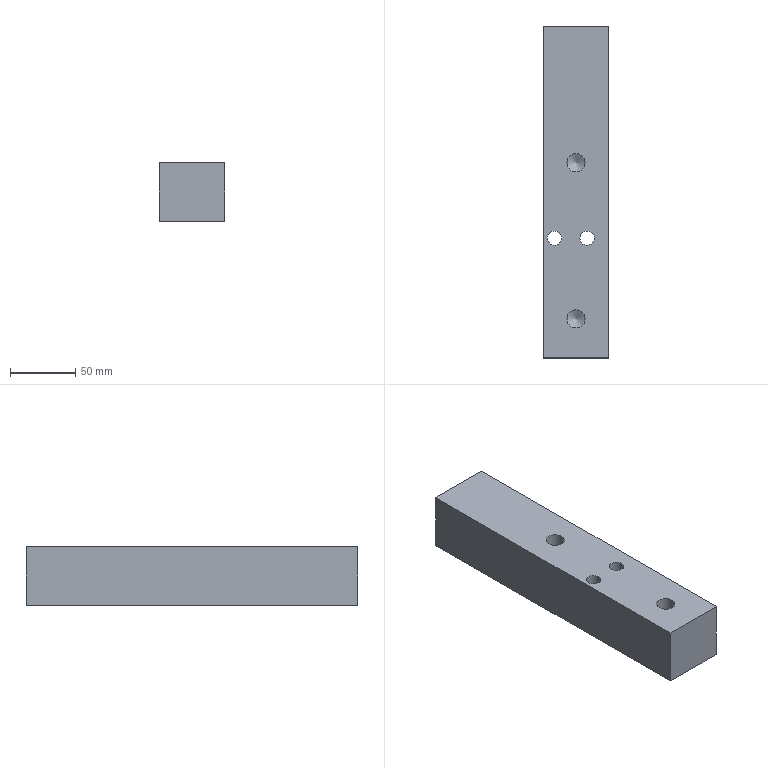Part | STEP file | 019_id2166_x_t | 1 solid | 14 faces | box 50 x 255 x 45 mm | volume 554819 mm3 | plane 6 | cylinder 5 | cone 3 | commonest cylinder face diameters 14 x3 11 x2
STEP:
#1=CARTESIAN_POINT('',(0.,0.,0.));
#2=DIRECTION('',(0.,0.,1.));
#3=DIRECTION('',(1.,0.,0.));
#4=AXIS2_PLACEMENT_3D('',#1,#2,#3);
#5=CARTESIAN_POINT('',(7.5,232.,185.));
#6=VERTEX_POINT('',#5);
#7=CARTESIAN_POINT('',(-3.5,232.,185.));
#8=VERTEX_POINT('',#7);
#9=CARTESIAN_POINT('',(2.,232.,185.));
#10=DIRECTION('',(0.,0.,1.));
#11=DIRECTION('',(1.,0.,0.));
#12=AXIS2_PLACEMENT_3D('',#9,#10,#11);
#13=CIRCLE('',#12,5.5);
#14=CARTESIAN_POINT('',(173.5,0.,185.));
#15=DIRECTION('',(0.,0.,-1.));
#16=DIRECTION('',(1.,0.,0.));
#17=AXIS2_PLACEMENT_3D('',#14,#15,#16);
#18=PLANE('',#17);
#19=CARTESIAN_POINT('',(-166.,-232.));
#20=CARTESIAN_POINT('',(-166.,-241.526));
#21=CARTESIAN_POINT('',(-174.25,-236.763));
#22=CARTESIAN_POINT('',(-182.5,-232.));
#23=CARTESIAN_POINT('',(-174.25,-227.237));
#24=CARTESIAN_POINT('',(-166.,-222.474));
#25=CARTESIAN_POINT('',(-166.,-232.));
#26=(BOUNDED_CURVE()B_SPLINE_CURVE(2,(#19,#20,#21,#22,#23,#24,#25),.UNSPECIFIED.,.T.,.F.)B_SPLINE_CURVE_WITH_KNOTS((1,2,2,2,2,1),(-2.094,0.,2.094,4.189,6.283,8.378),.UNSPECIFIED.)CURVE()GEOMETRIC_REPRESENTATION_ITEM()RATIONAL_B_SPLINE_CURVE((1.,0.5,1.,0.5,1.,0.5,1.))REPRESENTATION_ITEM(''));
#27=(GEOMETRIC_REPRESENTATION_CONTEXT(2)PARAMETRIC_REPRESENTATION_CONTEXT()REPRESENTATION_CONTEXT('',''));
#28=DEFINITIONAL_REPRESENTATION('',(#26),#27);
#29=PCURVE('',#18,#28);
#30=CARTESIAN_POINT('',(2.,232.,595.));
#31=DIRECTION('',(0.,0.,-1.));
#32=DIRECTION('',(-1.,0.,0.));
#33=AXIS2_PLACEMENT_3D('',#30,#31,#32);
#34=CYLINDRICAL_SURFACE('',#33,5.5);
#35=CARTESIAN_POINT('',(3.142,410.));
#36=DIRECTION('',(-1.,0.));
#37=VECTOR('',#36,1.);
#38=LINE('',#35,#37);
#39=(GEOMETRIC_REPRESENTATION_CONTEXT(2)PARAMETRIC_REPRESENTATION_CONTEXT()REPRESENTATION_CONTEXT('',''));
#40=DEFINITIONAL_REPRESENTATION('',(#38),#39);
#41=PCURVE('',#34,#40);
#42=SURFACE_CURVE('',#13,(#29,#41),.PCURVE_S1.);
#43=EDGE_CURVE('',#6,#8,#42,.T.);
#44=ORIENTED_EDGE('',*,*,#43,.T.);
#45=CARTESIAN_POINT('',(2.,232.,185.));
#46=DIRECTION('',(0.,0.,1.));
#47=DIRECTION('',(1.,0.,0.));
#48=AXIS2_PLACEMENT_3D('',#45,#46,#47);
#49=CIRCLE('',#48,5.5);
#50=CARTESIAN_POINT('',(-166.,-232.));
#51=CARTESIAN_POINT('',(-166.,-241.526));
#52=CARTESIAN_POINT('',(-174.25,-236.763));
#53=CARTESIAN_POINT('',(-182.5,-232.));
#54=CARTESIAN_POINT('',(-174.25,-227.237));
#55=CARTESIAN_POINT('',(-166.,-222.474));
#56=CARTESIAN_POINT('',(-166.,-232.));
#57=(BOUNDED_CURVE()B_SPLINE_CURVE(2,(#50,#51,#52,#53,#54,#55,#56),.UNSPECIFIED.,.T.,.F.)B_SPLINE_CURVE_WITH_KNOTS((1,2,2,2,2,1),(-2.094,0.,2.094,4.189,6.283,8.378),.UNSPECIFIED.)CURVE()GEOMETRIC_REPRESENTATION_ITEM()RATIONAL_B_SPLINE_CURVE((1.,0.5,1.,0.5,1.,0.5,1.))REPRESENTATION_ITEM(''));
#58=(GEOMETRIC_REPRESENTATION_CONTEXT(2)PARAMETRIC_REPRESENTATION_CONTEXT()REPRESENTATION_CONTEXT('',''));
#59=DEFINITIONAL_REPRESENTATION('',(#57),#58);
#60=PCURVE('',#18,#59);
#61=CARTESIAN_POINT('',(9.425,410.));
#62=DIRECTION('',(-1.,0.));
#63=VECTOR('',#62,1.);
#64=LINE('',#61,#63);
#65=(GEOMETRIC_REPRESENTATION_CONTEXT(2)PARAMETRIC_REPRESENTATION_CONTEXT()REPRESENTATION_CONTEXT('',''));
#66=DEFINITIONAL_REPRESENTATION('',(#64),#65);
#67=PCURVE('',#34,#66);
#68=SURFACE_CURVE('',#49,(#60,#67),.PCURVE_S1.);
#69=EDGE_CURVE('',#8,#6,#68,.T.);
#70=ORIENTED_EDGE('',*,*,#69,.T.);
#71=EDGE_LOOP('',(#44,#70));
#72=FACE_BOUND('',#71,.T.);
#73=CARTESIAN_POINT('',(-13.5,370.,185.));
#74=VERTEX_POINT('',#73);
#75=CARTESIAN_POINT('',(-6.5,370.,185.));
#76=DIRECTION('',(0.,0.,-1.));
#77=DIRECTION('',(-1.,0.,0.));
#78=AXIS2_PLACEMENT_3D('',#75,#76,#77);
#79=CIRCLE('',#78,7.);
#80=CARTESIAN_POINT('',(-180.,-370.));
#81=DIRECTION('',(-1.,0.));
#82=AXIS2_PLACEMENT_2D('',#80,#81);
#83=CIRCLE('',#82,7.);
#84=(GEOMETRIC_REPRESENTATION_CONTEXT(2)PARAMETRIC_REPRESENTATION_CONTEXT()REPRESENTATION_CONTEXT('',''));
#85=DEFINITIONAL_REPRESENTATION('',(#83),#84);
#86=PCURVE('',#18,#85);
#87=CARTESIAN_POINT('',(-6.5,370.,121.));
#88=DIRECTION('',(0.,0.,1.));
#89=DIRECTION('',(1.,0.,0.));
#90=AXIS2_PLACEMENT_3D('',#87,#88,#89);
#91=CYLINDRICAL_SURFACE('',#90,7.);
#92=CARTESIAN_POINT('',(9.425,64.));
#93=DIRECTION('',(-1.,0.));
#94=VECTOR('',#93,1.);
#95=LINE('',#92,#94);
#96=(GEOMETRIC_REPRESENTATION_CONTEXT(2)PARAMETRIC_REPRESENTATION_CONTEXT()REPRESENTATION_CONTEXT('',''));
#97=DEFINITIONAL_REPRESENTATION('',(#95),#96);
#98=PCURVE('',#91,#97);
#99=SURFACE_CURVE('',#79,(#86,#98),.PCURVE_S1.);
#100=EDGE_CURVE('',#74,#74,#99,.T.);
#101=ORIENTED_EDGE('',*,*,#100,.F.);
#102=EDGE_LOOP('',(#101));
#103=FACE_BOUND('',#102,.T.);
#104=CARTESIAN_POINT('',(18.5,395.,185.));
#105=VERTEX_POINT('',#104);
#106=CARTESIAN_POINT('',(18.5,140.,185.));
#107=VERTEX_POINT('',#106);
#108=CARTESIAN_POINT('',(18.5,-210.,185.));
#109=DIRECTION('',(0.,-1.,0.));
#110=VECTOR('',#109,1.);
#111=LINE('',#108,#110);
#112=CARTESIAN_POINT('',(-155.,210.));
#113=DIRECTION('',(0.,1.));
#114=VECTOR('',#113,1.);
#115=LINE('',#112,#114);
#116=(GEOMETRIC_REPRESENTATION_CONTEXT(2)PARAMETRIC_REPRESENTATION_CONTEXT()REPRESENTATION_CONTEXT('',''));
#117=DEFINITIONAL_REPRESENTATION('',(#115),#116);
#118=PCURVE('',#18,#117);
#119=CARTESIAN_POINT('',(18.5,-210.,-28.5));
#120=DIRECTION('',(-1.,0.,0.));
#121=DIRECTION('',(0.,0.,1.));
#122=AXIS2_PLACEMENT_3D('',#119,#120,#121);
#123=PLANE('',#122);
#124=CARTESIAN_POINT('',(213.5,0.));
#125=DIRECTION('',(0.,-1.));
#126=VECTOR('',#125,1.);
#127=LINE('',#124,#126);
#128=(GEOMETRIC_REPRESENTATION_CONTEXT(2)PARAMETRIC_REPRESENTATION_CONTEXT()REPRESENTATION_CONTEXT('',''));
#129=DEFINITIONAL_REPRESENTATION('',(#127),#128);
#130=PCURVE('',#123,#129);
#131=SURFACE_CURVE('',#111,(#118,#130),.PCURVE_S1.);
#132=EDGE_CURVE('',#105,#107,#131,.T.);
#133=ORIENTED_EDGE('',*,*,#132,.T.);
#134=CARTESIAN_POINT('',(-31.5,140.,185.));
#135=VERTEX_POINT('',#134);
#136=CARTESIAN_POINT('',(513.5,140.,185.));
#137=DIRECTION('',(-1.,0.,0.));
#138=VECTOR('',#137,1.);
#139=LINE('',#136,#138);
#140=CARTESIAN_POINT('',(340.,-140.));
#141=DIRECTION('',(-1.,0.));
#142=VECTOR('',#141,1.);
#143=LINE('',#140,#142);
#144=(GEOMETRIC_REPRESENTATION_CONTEXT(2)PARAMETRIC_REPRESENTATION_CONTEXT()REPRESENTATION_CONTEXT('',''));
#145=DEFINITIONAL_REPRESENTATION('',(#143),#144);
#146=PCURVE('',#18,#145);
#147=CARTESIAN_POINT('',(513.5,140.,428.5));
#148=DIRECTION('',(0.,1.,0.));
#149=DIRECTION('',(0.,0.,-1.));
#150=AXIS2_PLACEMENT_3D('',#147,#148,#149);
#151=PLANE('',#150);
#152=CARTESIAN_POINT('',(243.5,0.));
#153=DIRECTION('',(0.,1.));
#154=VECTOR('',#153,1.);
#155=LINE('',#152,#154);
#156=(GEOMETRIC_REPRESENTATION_CONTEXT(2)PARAMETRIC_REPRESENTATION_CONTEXT()REPRESENTATION_CONTEXT('',''));
#157=DEFINITIONAL_REPRESENTATION('',(#155),#156);
#158=PCURVE('',#151,#157);
#159=SURFACE_CURVE('',#139,(#146,#158),.PCURVE_S1.);
#160=EDGE_CURVE('',#107,#135,#159,.T.);
#161=ORIENTED_EDGE('',*,*,#160,.T.);
#162=CARTESIAN_POINT('',(-31.5,395.,185.));
#163=VERTEX_POINT('',#162);
#164=CARTESIAN_POINT('',(-31.5,0.,185.));
#165=DIRECTION('',(0.,1.,0.));
#166=VECTOR('',#165,1.);
#167=LINE('',#164,#166);
#168=CARTESIAN_POINT('',(-205.,0.));
#169=DIRECTION('',(0.,-1.));
#170=VECTOR('',#169,1.);
#171=LINE('',#168,#170);
#172=(GEOMETRIC_REPRESENTATION_CONTEXT(2)PARAMETRIC_REPRESENTATION_CONTEXT()REPRESENTATION_CONTEXT('',''));
#173=DEFINITIONAL_REPRESENTATION('',(#171),#172);
#174=PCURVE('',#18,#173);
#175=CARTESIAN_POINT('',(-31.5,-210.,-28.5));
#176=DIRECTION('',(-1.,0.,0.));
#177=DIRECTION('',(0.,0.,1.));
#178=AXIS2_PLACEMENT_3D('',#175,#176,#177);
#179=PLANE('',#178);
#180=CARTESIAN_POINT('',(213.5,210.));
#181=DIRECTION('',(0.,1.));
#182=VECTOR('',#181,1.);
#183=LINE('',#180,#182);
#184=(GEOMETRIC_REPRESENTATION_CONTEXT(2)PARAMETRIC_REPRESENTATION_CONTEXT()REPRESENTATION_CONTEXT('',''));
#185=DEFINITIONAL_REPRESENTATION('',(#183),#184);
#186=PCURVE('',#179,#185);
#187=SURFACE_CURVE('',#167,(#174,#186),.PCURVE_S1.);
#188=EDGE_CURVE('',#135,#163,#187,.T.);
#189=ORIENTED_EDGE('',*,*,#188,.T.);
#190=CARTESIAN_POINT('',(173.5,395.,185.));
#191=DIRECTION('',(1.,0.,0.));
#192=VECTOR('',#191,1.);
#193=LINE('',#190,#192);
#194=CARTESIAN_POINT('',(0.,-395.));
#195=DIRECTION('',(1.,0.));
#196=VECTOR('',#195,1.);
#197=LINE('',#194,#196);
#198=(GEOMETRIC_REPRESENTATION_CONTEXT(2)PARAMETRIC_REPRESENTATION_CONTEXT()REPRESENTATION_CONTEXT('',''));
#199=DEFINITIONAL_REPRESENTATION('',(#197),#198);
#200=PCURVE('',#18,#199);
#201=CARTESIAN_POINT('',(-31.5,395.,-28.5));
#202=DIRECTION('',(0.,1.,0.));
#203=DIRECTION('',(0.,0.,-1.));
#204=AXIS2_PLACEMENT_3D('',#201,#202,#203);
#205=PLANE('',#204);
#206=CARTESIAN_POINT('',(-213.5,-205.));
#207=DIRECTION('',(0.,-1.));
#208=VECTOR('',#207,1.);
#209=LINE('',#206,#208);
#210=(GEOMETRIC_REPRESENTATION_CONTEXT(2)PARAMETRIC_REPRESENTATION_CONTEXT()REPRESENTATION_CONTEXT('',''));
#211=DEFINITIONAL_REPRESENTATION('',(#209),#210);
#212=PCURVE('',#205,#211);
#213=SURFACE_CURVE('',#193,(#200,#212),.PCURVE_S1.);
#214=EDGE_CURVE('',#163,#105,#213,.T.);
#215=ORIENTED_EDGE('',*,*,#214,.T.);
#216=EDGE_LOOP('',(#133,#161,#189,#215));
#217=FACE_BOUND('',#216,.T.);
#218=CARTESIAN_POINT('',(-17.5,232.,185.));
#219=VERTEX_POINT('',#218);
#220=CARTESIAN_POINT('',(-28.5,232.,185.));
#221=VERTEX_POINT('',#220);
#222=CARTESIAN_POINT('',(-23.,232.,185.));
#223=DIRECTION('',(0.,0.,1.));
#224=DIRECTION('',(1.,0.,0.));
#225=AXIS2_PLACEMENT_3D('',#222,#223,#224);
#226=CIRCLE('',#225,5.5);
#227=CARTESIAN_POINT('',(-191.,-232.));
#228=CARTESIAN_POINT('',(-191.,-241.526));
#229=CARTESIAN_POINT('',(-199.25,-236.763));
#230=CARTESIAN_POINT('',(-207.5,-232.));
#231=CARTESIAN_POINT('',(-199.25,-227.237));
#232=CARTESIAN_POINT('',(-191.,-222.474));
#233=CARTESIAN_POINT('',(-191.,-232.));
#234=(BOUNDED_CURVE()B_SPLINE_CURVE(2,(#227,#228,#229,#230,#231,#232,#233),.UNSPECIFIED.,.T.,.F.)B_SPLINE_CURVE_WITH_KNOTS((1,2,2,2,2,1),(-2.094,0.,2.094,4.189,6.283,8.378),.UNSPECIFIED.)CURVE()GEOMETRIC_REPRESENTATION_ITEM()RATIONAL_B_SPLINE_CURVE((1.,0.5,1.,0.5,1.,0.5,1.))REPRESENTATION_ITEM(''));
#235=(GEOMETRIC_REPRESENTATION_CONTEXT(2)PARAMETRIC_REPRESENTATION_CONTEXT()REPRESENTATION_CONTEXT('',''));
#236=DEFINITIONAL_REPRESENTATION('',(#234),#235);
#237=PCURVE('',#18,#236);
#238=CARTESIAN_POINT('',(-23.,232.,595.));
#239=DIRECTION('',(0.,0.,-1.));
#240=DIRECTION('',(-1.,0.,0.));
#241=AXIS2_PLACEMENT_3D('',#238,#239,#240);
#242=CYLINDRICAL_SURFACE('',#241,5.5);
#243=CARTESIAN_POINT('',(3.142,410.));
#244=DIRECTION('',(-1.,0.));
#245=VECTOR('',#244,1.);
#246=LINE('',#243,#245);
#247=(GEOMETRIC_REPRESENTATION_CONTEXT(2)PARAMETRIC_REPRESENTATION_CONTEXT()REPRESENTATION_CONTEXT('',''));
#248=DEFINITIONAL_REPRESENTATION('',(#246),#247);
#249=PCURVE('',#242,#248);
#250=SURFACE_CURVE('',#226,(#237,#249),.PCURVE_S1.);
#251=EDGE_CURVE('',#219,#221,#250,.T.);
#252=ORIENTED_EDGE('',*,*,#251,.T.);
#253=CARTESIAN_POINT('',(-23.,232.,185.));
#254=DIRECTION('',(0.,0.,1.));
#255=DIRECTION('',(1.,0.,0.));
#256=AXIS2_PLACEMENT_3D('',#253,#254,#255);
#257=CIRCLE('',#256,5.5);
#258=CARTESIAN_POINT('',(-191.,-232.));
#259=CARTESIAN_POINT('',(-191.,-241.526));
#260=CARTESIAN_POINT('',(-199.25,-236.763));
#261=CARTESIAN_POINT('',(-207.5,-232.));
#262=CARTESIAN_POINT('',(-199.25,-227.237));
#263=CARTESIAN_POINT('',(-191.,-222.474));
#264=CARTESIAN_POINT('',(-191.,-232.));
#265=(BOUNDED_CURVE()B_SPLINE_CURVE(2,(#258,#259,#260,#261,#262,#263,#264),.UNSPECIFIED.,.T.,.F.)B_SPLINE_CURVE_WITH_KNOTS((1,2,2,2,2,1),(-2.094,0.,2.094,4.189,6.283,8.378),.UNSPECIFIED.)CURVE()GEOMETRIC_REPRESENTATION_ITEM()RATIONAL_B_SPLINE_CURVE((1.,0.5,1.,0.5,1.,0.5,1.))REPRESENTATION_ITEM(''));
#266=(GEOMETRIC_REPRESENTATION_CONTEXT(2)PARAMETRIC_REPRESENTATION_CONTEXT()REPRESENTATION_CONTEXT('',''));
#267=DEFINITIONAL_REPRESENTATION('',(#265),#266);
#268=PCURVE('',#18,#267);
#269=CARTESIAN_POINT('',(9.425,410.));
#270=DIRECTION('',(-1.,0.));
#271=VECTOR('',#270,1.);
#272=LINE('',#269,#271);
#273=(GEOMETRIC_REPRESENTATION_CONTEXT(2)PARAMETRIC_REPRESENTATION_CONTEXT()REPRESENTATION_CONTEXT('',''));
#274=DEFINITIONAL_REPRESENTATION('',(#272),#273);
#275=PCURVE('',#242,#274);
#276=SURFACE_CURVE('',#257,(#268,#275),.PCURVE_S1.);
#277=EDGE_CURVE('',#221,#219,#276,.T.);
#278=ORIENTED_EDGE('',*,*,#277,.T.);
#279=EDGE_LOOP('',(#252,#278));
#280=FACE_BOUND('',#279,.T.);
#281=ADVANCED_FACE('',(#72,#103,#217,#280),#18,.T.);
#282=CARTESIAN_POINT('',(-3.5,232.,230.));
#283=VERTEX_POINT('',#282);
#284=CARTESIAN_POINT('',(2.,232.,230.));
#285=DIRECTION('',(0.,0.,1.));
#286=DIRECTION('',(-1.,0.,0.));
#287=AXIS2_PLACEMENT_3D('',#284,#285,#286);
#288=CIRCLE('',#287,5.5);
#289=CARTESIAN_POINT('',(-31.5,-210.,230.));
#290=DIRECTION('',(0.,0.,-1.));
#291=DIRECTION('',(0.,-1.,0.));
#292=AXIS2_PLACEMENT_3D('',#289,#290,#291);
#293=PLANE('',#292);
#294=CARTESIAN_POINT('',(-442.,-28.));
#295=CARTESIAN_POINT('',(-432.474,-28.));
#296=CARTESIAN_POINT('',(-437.237,-36.25));
#297=CARTESIAN_POINT('',(-442.,-44.5));
#298=CARTESIAN_POINT('',(-446.763,-36.25));
#299=CARTESIAN_POINT('',(-451.526,-28.));
#300=CARTESIAN_POINT('',(-442.,-28.));
#301=(BOUNDED_CURVE()B_SPLINE_CURVE(2,(#294,#295,#296,#297,#298,#299,#300),.UNSPECIFIED.,.T.,.F.)B_SPLINE_CURVE_WITH_KNOTS((1,2,2,2,2,1),(-2.094,0.,2.094,4.189,6.283,8.378),.UNSPECIFIED.)CURVE()GEOMETRIC_REPRESENTATION_ITEM()RATIONAL_B_SPLINE_CURVE((1.,0.5,1.,0.5,1.,0.5,1.))REPRESENTATION_ITEM(''));
#302=(GEOMETRIC_REPRESENTATION_CONTEXT(2)PARAMETRIC_REPRESENTATION_CONTEXT()REPRESENTATION_CONTEXT('',''));
#303=DEFINITIONAL_REPRESENTATION('',(#301),#302);
#304=PCURVE('',#293,#303);
#305=CARTESIAN_POINT('',(6.283,365.));
#306=DIRECTION('',(-1.,0.));
#307=VECTOR('',#306,1.);
#308=LINE('',#305,#307);
#309=(GEOMETRIC_REPRESENTATION_CONTEXT(2)PARAMETRIC_REPRESENTATION_CONTEXT()REPRESENTATION_CONTEXT('',''));
#310=DEFINITIONAL_REPRESENTATION('',(#308),#309);
#311=PCURVE('',#34,#310);
#312=SURFACE_CURVE('',#288,(#304,#311),.PCURVE_S1.);
#313=EDGE_CURVE('',#283,#283,#312,.T.);
#314=ORIENTED_EDGE('',*,*,#313,.F.);
#315=EDGE_LOOP('',(#314));
#316=FACE_BOUND('',#315,.T.);
#317=CARTESIAN_POINT('',(-13.5,170.,230.));
#318=VERTEX_POINT('',#317);
#319=CARTESIAN_POINT('',(-6.5,170.,230.));
#320=DIRECTION('',(0.,0.,-1.));
#321=DIRECTION('',(-1.,0.,0.));
#322=AXIS2_PLACEMENT_3D('',#319,#320,#321);
#323=CIRCLE('',#322,7.);
#324=CARTESIAN_POINT('',(-380.,-25.));
#325=DIRECTION('',(0.,1.));
#326=AXIS2_PLACEMENT_2D('',#324,#325);
#327=CIRCLE('',#326,7.);
#328=(GEOMETRIC_REPRESENTATION_CONTEXT(2)PARAMETRIC_REPRESENTATION_CONTEXT()REPRESENTATION_CONTEXT('',''));
#329=DEFINITIONAL_REPRESENTATION('',(#327),#328);
#330=PCURVE('',#293,#329);
#331=CARTESIAN_POINT('',(-6.5,170.,279.));
#332=DIRECTION('',(0.,0.,-1.));
#333=DIRECTION('',(1.,0.,0.));
#334=AXIS2_PLACEMENT_3D('',#331,#332,#333);
#335=CYLINDRICAL_SURFACE('',#334,7.);
#336=CARTESIAN_POINT('',(3.142,49.));
#337=DIRECTION('',(1.,0.));
#338=VECTOR('',#337,1.);
#339=LINE('',#336,#338);
#340=(GEOMETRIC_REPRESENTATION_CONTEXT(2)PARAMETRIC_REPRESENTATION_CONTEXT()REPRESENTATION_CONTEXT('',''));
#341=DEFINITIONAL_REPRESENTATION('',(#339),#340);
#342=PCURVE('',#335,#341);
#343=SURFACE_CURVE('',#323,(#330,#342),.PCURVE_S1.);
#344=EDGE_CURVE('',#318,#318,#343,.T.);
#345=ORIENTED_EDGE('',*,*,#344,.T.);
#346=EDGE_LOOP('',(#345));
#347=FACE_BOUND('',#346,.T.);
#348=CARTESIAN_POINT('',(-13.5,290.,230.));
#349=VERTEX_POINT('',#348);
#350=CARTESIAN_POINT('',(-6.5,290.,230.));
#351=DIRECTION('',(0.,0.,-1.));
#352=DIRECTION('',(-1.,0.,0.));
#353=AXIS2_PLACEMENT_3D('',#350,#351,#352);
#354=CIRCLE('',#353,7.);
#355=CARTESIAN_POINT('',(-500.,-25.));
#356=DIRECTION('',(0.,1.));
#357=AXIS2_PLACEMENT_2D('',#355,#356);
#358=CIRCLE('',#357,7.);
#359=(GEOMETRIC_REPRESENTATION_CONTEXT(2)PARAMETRIC_REPRESENTATION_CONTEXT()REPRESENTATION_CONTEXT('',''));
#360=DEFINITIONAL_REPRESENTATION('',(#358),#359);
#361=PCURVE('',#293,#360);
#362=CARTESIAN_POINT('',(-6.5,290.,279.));
#363=DIRECTION('',(0.,0.,-1.));
#364=DIRECTION('',(1.,0.,0.));
#365=AXIS2_PLACEMENT_3D('',#362,#363,#364);
#366=CYLINDRICAL_SURFACE('',#365,7.);
#367=CARTESIAN_POINT('',(3.142,49.));
#368=DIRECTION('',(1.,0.));
#369=VECTOR('',#368,1.);
#370=LINE('',#367,#369);
#371=(GEOMETRIC_REPRESENTATION_CONTEXT(2)PARAMETRIC_REPRESENTATION_CONTEXT()REPRESENTATION_CONTEXT('',''));
#372=DEFINITIONAL_REPRESENTATION('',(#370),#371);
#373=PCURVE('',#366,#372);
#374=SURFACE_CURVE('',#354,(#361,#373),.PCURVE_S1.);
#375=EDGE_CURVE('',#349,#349,#374,.T.);
#376=ORIENTED_EDGE('',*,*,#375,.T.);
#377=EDGE_LOOP('',(#376));
#378=FACE_BOUND('',#377,.T.);
#379=CARTESIAN_POINT('',(-31.5,395.,230.));
#380=VERTEX_POINT('',#379);
#381=CARTESIAN_POINT('',(-31.5,140.,230.));
#382=VERTEX_POINT('',#381);
#383=CARTESIAN_POINT('',(-31.5,-210.,230.));
#384=DIRECTION('',(0.,-1.,0.));
#385=VECTOR('',#384,1.);
#386=LINE('',#383,#385);
#387=CARTESIAN_POINT('',(0.,0.));
#388=DIRECTION('',(1.,0.));
#389=VECTOR('',#388,1.);
#390=LINE('',#387,#389);
#391=(GEOMETRIC_REPRESENTATION_CONTEXT(2)PARAMETRIC_REPRESENTATION_CONTEXT()REPRESENTATION_CONTEXT('',''));
#392=DEFINITIONAL_REPRESENTATION('',(#390),#391);
#393=PCURVE('',#293,#392);
#394=CARTESIAN_POINT('',(258.5,0.));
#395=DIRECTION('',(0.,-1.));
#396=VECTOR('',#395,1.);
#397=LINE('',#394,#396);
#398=(GEOMETRIC_REPRESENTATION_CONTEXT(2)PARAMETRIC_REPRESENTATION_CONTEXT()REPRESENTATION_CONTEXT('',''));
#399=DEFINITIONAL_REPRESENTATION('',(#397),#398);
#400=PCURVE('',#179,#399);
#401=SURFACE_CURVE('',#386,(#393,#400),.PCURVE_S1.);
#402=EDGE_CURVE('',#380,#382,#401,.T.);
#403=ORIENTED_EDGE('',*,*,#402,.T.);
#404=CARTESIAN_POINT('',(18.5,140.,230.));
#405=VERTEX_POINT('',#404);
#406=CARTESIAN_POINT('',(-31.5,140.,230.));
#407=DIRECTION('',(1.,0.,0.));
#408=VECTOR('',#407,1.);
#409=LINE('',#406,#408);
#410=CARTESIAN_POINT('',(-350.,0.));
#411=DIRECTION('',(0.,-1.));
#412=VECTOR('',#411,1.);
#413=LINE('',#410,#412);
#414=(GEOMETRIC_REPRESENTATION_CONTEXT(2)PARAMETRIC_REPRESENTATION_CONTEXT()REPRESENTATION_CONTEXT('',''));
#415=DEFINITIONAL_REPRESENTATION('',(#413),#414);
#416=PCURVE('',#293,#415);
#417=CARTESIAN_POINT('',(198.5,545.));
#418=DIRECTION('',(0.,-1.));
#419=VECTOR('',#418,1.);
#420=LINE('',#417,#419);
#421=(GEOMETRIC_REPRESENTATION_CONTEXT(2)PARAMETRIC_REPRESENTATION_CONTEXT()REPRESENTATION_CONTEXT('',''));
#422=DEFINITIONAL_REPRESENTATION('',(#420),#421);
#423=PCURVE('',#151,#422);
#424=SURFACE_CURVE('',#409,(#416,#423),.PCURVE_S1.);
#425=EDGE_CURVE('',#382,#405,#424,.T.);
#426=ORIENTED_EDGE('',*,*,#425,.T.);
#427=CARTESIAN_POINT('',(18.5,395.,230.));
#428=VERTEX_POINT('',#427);
#429=CARTESIAN_POINT('',(18.5,-210.,230.));
#430=DIRECTION('',(0.,-1.,0.));
#431=VECTOR('',#430,1.);
#432=LINE('',#429,#431);
#433=CARTESIAN_POINT('',(0.,-50.));
#434=DIRECTION('',(1.,0.));
#435=VECTOR('',#434,1.);
#436=LINE('',#433,#435);
#437=(GEOMETRIC_REPRESENTATION_CONTEXT(2)PARAMETRIC_REPRESENTATION_CONTEXT()REPRESENTATION_CONTEXT('',''));
#438=DEFINITIONAL_REPRESENTATION('',(#436),#437);
#439=PCURVE('',#293,#438);
#440=CARTESIAN_POINT('',(258.5,0.));
#441=DIRECTION('',(0.,-1.));
#442=VECTOR('',#441,1.);
#443=LINE('',#440,#442);
#444=(GEOMETRIC_REPRESENTATION_CONTEXT(2)PARAMETRIC_REPRESENTATION_CONTEXT()REPRESENTATION_CONTEXT('',''));
#445=DEFINITIONAL_REPRESENTATION('',(#443),#444);
#446=PCURVE('',#123,#445);
#447=SURFACE_CURVE('',#432,(#439,#446),.PCURVE_S1.);
#448=EDGE_CURVE('',#428,#405,#447,.T.);
#449=ORIENTED_EDGE('',*,*,#448,.F.);
#450=CARTESIAN_POINT('',(-31.5,395.,230.));
#451=DIRECTION('',(1.,0.,0.));
#452=VECTOR('',#451,1.);
#453=LINE('',#450,#452);
#454=CARTESIAN_POINT('',(-605.,0.));
#455=DIRECTION('',(0.,-1.));
#456=VECTOR('',#455,1.);
#457=LINE('',#454,#456);
#458=(GEOMETRIC_REPRESENTATION_CONTEXT(2)PARAMETRIC_REPRESENTATION_CONTEXT()REPRESENTATION_CONTEXT('',''));
#459=DEFINITIONAL_REPRESENTATION('',(#457),#458);
#460=PCURVE('',#293,#459);
#461=CARTESIAN_POINT('',(-258.5,0.));
#462=DIRECTION('',(0.,-1.));
#463=VECTOR('',#462,1.);
#464=LINE('',#461,#463);
#465=(GEOMETRIC_REPRESENTATION_CONTEXT(2)PARAMETRIC_REPRESENTATION_CONTEXT()REPRESENTATION_CONTEXT('',''));
#466=DEFINITIONAL_REPRESENTATION('',(#464),#465);
#467=PCURVE('',#205,#466);
#468=SURFACE_CURVE('',#453,(#460,#467),.PCURVE_S1.);
#469=EDGE_CURVE('',#380,#428,#468,.T.);
#470=ORIENTED_EDGE('',*,*,#469,.F.);
#471=EDGE_LOOP('',(#403,#426,#449,#470));
#472=FACE_BOUND('',#471,.T.);
#473=CARTESIAN_POINT('',(-28.5,232.,230.));
#474=VERTEX_POINT('',#473);
#475=CARTESIAN_POINT('',(-23.,232.,230.));
#476=DIRECTION('',(0.,0.,1.));
#477=DIRECTION('',(-1.,0.,0.));
#478=AXIS2_PLACEMENT_3D('',#475,#476,#477);
#479=CIRCLE('',#478,5.5);
#480=CARTESIAN_POINT('',(-442.,-3.));
#481=CARTESIAN_POINT('',(-432.474,-3.));
#482=CARTESIAN_POINT('',(-437.237,-11.25));
#483=CARTESIAN_POINT('',(-442.,-19.5));
#484=CARTESIAN_POINT('',(-446.763,-11.25));
#485=CARTESIAN_POINT('',(-451.526,-3.));
#486=CARTESIAN_POINT('',(-442.,-3.));
#487=(BOUNDED_CURVE()B_SPLINE_CURVE(2,(#480,#481,#482,#483,#484,#485,#486),.UNSPECIFIED.,.T.,.F.)B_SPLINE_CURVE_WITH_KNOTS((1,2,2,2,2,1),(-2.094,0.,2.094,4.189,6.283,8.378),.UNSPECIFIED.)CURVE()GEOMETRIC_REPRESENTATION_ITEM()RATIONAL_B_SPLINE_CURVE((1.,0.5,1.,0.5,1.,0.5,1.))REPRESENTATION_ITEM(''));
#488=(GEOMETRIC_REPRESENTATION_CONTEXT(2)PARAMETRIC_REPRESENTATION_CONTEXT()REPRESENTATION_CONTEXT('',''));
#489=DEFINITIONAL_REPRESENTATION('',(#487),#488);
#490=PCURVE('',#293,#489);
#491=CARTESIAN_POINT('',(6.283,365.));
#492=DIRECTION('',(-1.,0.));
#493=VECTOR('',#492,1.);
#494=LINE('',#491,#493);
#495=(GEOMETRIC_REPRESENTATION_CONTEXT(2)PARAMETRIC_REPRESENTATION_CONTEXT()REPRESENTATION_CONTEXT('',''));
#496=DEFINITIONAL_REPRESENTATION('',(#494),#495);
#497=PCURVE('',#242,#496);
#498=SURFACE_CURVE('',#479,(#490,#497),.PCURVE_S1.);
#499=EDGE_CURVE('',#474,#474,#498,.T.);
#500=ORIENTED_EDGE('',*,*,#499,.F.);
#501=EDGE_LOOP('',(#500));
#502=FACE_BOUND('',#501,.T.);
#503=ADVANCED_FACE('',(#316,#347,#378,#472,#502),#293,.F.);
#504=CARTESIAN_POINT('',(-6.5,170.,206.5));
#505=VERTEX_POINT('',#504);
#506=CARTESIAN_POINT('',(-13.5,170.,210.541));
#507=VERTEX_POINT('',#506);
#508=CARTESIAN_POINT('',(-6.5,170.,206.5));
#509=CARTESIAN_POINT('',(-13.5,170.,210.541));
#510=B_SPLINE_CURVE_WITH_KNOTS('',1,(#508,#509),.UNSPECIFIED.,.F.,.F.,(2,2),(-8.083,0.),.PIECEWISE_BEZIER_KNOTS.);
#511=CARTESIAN_POINT('',(-6.5,170.,210.541));
#512=DIRECTION('',(0.,0.,1.));
#513=DIRECTION('',(-1.,0.,0.));
#514=AXIS2_PLACEMENT_3D('',#511,#512,#513);
#515=CONICAL_SURFACE('',#514,7.,1.047);
#516=CARTESIAN_POINT('',(6.283,0.));
#517=DIRECTION('',(0.,1.));
#518=VECTOR('',#517,1.);
#519=LINE('',#516,#518);
#520=(GEOMETRIC_REPRESENTATION_CONTEXT(2)PARAMETRIC_REPRESENTATION_CONTEXT()REPRESENTATION_CONTEXT('',''));
#521=DEFINITIONAL_REPRESENTATION('',(#519),#520);
#522=PCURVE('',#515,#521);
#523=CARTESIAN_POINT('',(0.,0.));
#524=DIRECTION('',(0.,1.));
#525=VECTOR('',#524,1.);
#526=LINE('',#523,#525);
#527=(GEOMETRIC_REPRESENTATION_CONTEXT(2)PARAMETRIC_REPRESENTATION_CONTEXT()REPRESENTATION_CONTEXT('',''));
#528=DEFINITIONAL_REPRESENTATION('',(#526),#527);
#529=PCURVE('',#515,#528);
#530=SEAM_CURVE('',#510,(#522,#529),.PCURVE_S1.);
#531=EDGE_CURVE('',#505,#507,#530,.T.);
#532=ORIENTED_EDGE('',*,*,#531,.T.);
#533=CARTESIAN_POINT('',(0.5,170.,210.541));
#534=VERTEX_POINT('',#533);
#535=CARTESIAN_POINT('',(-6.5,170.,210.541));
#536=DIRECTION('',(0.,0.,-1.));
#537=DIRECTION('',(1.,0.,0.));
#538=AXIS2_PLACEMENT_3D('',#535,#536,#537);
#539=CIRCLE('',#538,7.);
#540=CARTESIAN_POINT('',(9.425,0.));
#541=DIRECTION('',(-1.,0.));
#542=VECTOR('',#541,1.);
#543=LINE('',#540,#542);
#544=(GEOMETRIC_REPRESENTATION_CONTEXT(2)PARAMETRIC_REPRESENTATION_CONTEXT()REPRESENTATION_CONTEXT('',''));
#545=DEFINITIONAL_REPRESENTATION('',(#543),#544);
#546=PCURVE('',#515,#545);
#547=CARTESIAN_POINT('',(0.,68.459));
#548=DIRECTION('',(1.,0.));
#549=VECTOR('',#548,1.);
#550=LINE('',#547,#549);
#551=(GEOMETRIC_REPRESENTATION_CONTEXT(2)PARAMETRIC_REPRESENTATION_CONTEXT()REPRESENTATION_CONTEXT('',''));
#552=DEFINITIONAL_REPRESENTATION('',(#550),#551);
#553=PCURVE('',#335,#552);
#554=SURFACE_CURVE('',#539,(#546,#553),.PCURVE_S1.);
#555=EDGE_CURVE('',#507,#534,#554,.T.);
#556=ORIENTED_EDGE('',*,*,#555,.T.);
#557=CARTESIAN_POINT('',(-6.5,170.,210.541));
#558=DIRECTION('',(0.,0.,-1.));
#559=DIRECTION('',(1.,0.,0.));
#560=AXIS2_PLACEMENT_3D('',#557,#558,#559);
#561=CIRCLE('',#560,7.);
#562=CARTESIAN_POINT('',(3.142,0.));
#563=DIRECTION('',(-1.,0.));
#564=VECTOR('',#563,1.);
#565=LINE('',#562,#564);
#566=(GEOMETRIC_REPRESENTATION_CONTEXT(2)PARAMETRIC_REPRESENTATION_CONTEXT()REPRESENTATION_CONTEXT('',''));
#567=DEFINITIONAL_REPRESENTATION('',(#565),#566);
#568=PCURVE('',#515,#567);
#569=CARTESIAN_POINT('',(6.283,68.459));
#570=DIRECTION('',(1.,0.));
#571=VECTOR('',#570,1.);
#572=LINE('',#569,#571);
#573=(GEOMETRIC_REPRESENTATION_CONTEXT(2)PARAMETRIC_REPRESENTATION_CONTEXT()REPRESENTATION_CONTEXT('',''));
#574=DEFINITIONAL_REPRESENTATION('',(#572),#573);
#575=PCURVE('',#335,#574);
#576=SURFACE_CURVE('',#561,(#568,#575),.PCURVE_S1.);
#577=EDGE_CURVE('',#534,#507,#576,.T.);
#578=ORIENTED_EDGE('',*,*,#577,.T.);
#579=ORIENTED_EDGE('',*,*,#531,.F.);
#580=EDGE_LOOP('',(#532,#556,#578,#579));
#581=FACE_BOUND('',#580,.F.);
#582=ADVANCED_FACE('',(#581),#515,.F.);
#583=ORIENTED_EDGE('',*,*,#344,.T.);
#584=CARTESIAN_POINT('',(-13.5,170.,230.));
#585=CARTESIAN_POINT('',(-13.5,170.,210.541));
#586=B_SPLINE_CURVE_WITH_KNOTS('',1,(#584,#585),.UNSPECIFIED.,.F.,.F.,(2,2),(49.,68.459),.PIECEWISE_BEZIER_KNOTS.);
#587=CARTESIAN_POINT('',(9.425,0.));
#588=DIRECTION('',(0.,1.));
#589=VECTOR('',#588,1.);
#590=LINE('',#587,#589);
#591=(GEOMETRIC_REPRESENTATION_CONTEXT(2)PARAMETRIC_REPRESENTATION_CONTEXT()REPRESENTATION_CONTEXT('',''));
#592=DEFINITIONAL_REPRESENTATION('',(#590),#591);
#593=PCURVE('',#335,#592);
#594=CARTESIAN_POINT('',(3.142,0.));
#595=DIRECTION('',(0.,1.));
#596=VECTOR('',#595,1.);
#597=LINE('',#594,#596);
#598=(GEOMETRIC_REPRESENTATION_CONTEXT(2)PARAMETRIC_REPRESENTATION_CONTEXT()REPRESENTATION_CONTEXT('',''));
#599=DEFINITIONAL_REPRESENTATION('',(#597),#598);
#600=PCURVE('',#335,#599);
#601=SEAM_CURVE('',#586,(#593,#600),.PCURVE_S1.);
#602=EDGE_CURVE('',#318,#507,#601,.T.);
#603=ORIENTED_EDGE('',*,*,#602,.T.);
#604=ORIENTED_EDGE('',*,*,#577,.F.);
#605=ORIENTED_EDGE('',*,*,#555,.F.);
#606=ORIENTED_EDGE('',*,*,#602,.F.);
#607=EDGE_LOOP('',(#583,#603,#604,#605,#606));
#608=FACE_BOUND('',#607,.F.);
#609=ADVANCED_FACE('',(#608),#335,.F.);
#610=CARTESIAN_POINT('',(-6.5,370.,213.5));
#611=VERTEX_POINT('',#610);
#612=CARTESIAN_POINT('',(-13.5,370.,209.459));
#613=VERTEX_POINT('',#612);
#614=CARTESIAN_POINT('',(-6.5,370.,213.5));
#615=CARTESIAN_POINT('',(-13.5,370.,209.459));
#616=B_SPLINE_CURVE_WITH_KNOTS('',1,(#614,#615),.UNSPECIFIED.,.F.,.F.,(2,2),(-8.083,0.),.PIECEWISE_BEZIER_KNOTS.);
#617=CARTESIAN_POINT('',(-6.5,370.,209.459));
#618=DIRECTION('',(0.,0.,-1.));
#619=DIRECTION('',(-1.,0.,0.));
#620=AXIS2_PLACEMENT_3D('',#617,#618,#619);
#621=CONICAL_SURFACE('',#620,7.,1.047);
#622=CARTESIAN_POINT('',(6.283,0.));
#623=DIRECTION('',(0.,1.));
#624=VECTOR('',#623,1.);
#625=LINE('',#622,#624);
#626=(GEOMETRIC_REPRESENTATION_CONTEXT(2)PARAMETRIC_REPRESENTATION_CONTEXT()REPRESENTATION_CONTEXT('',''));
#627=DEFINITIONAL_REPRESENTATION('',(#625),#626);
#628=PCURVE('',#621,#627);
#629=CARTESIAN_POINT('',(0.,0.));
#630=DIRECTION('',(0.,1.));
#631=VECTOR('',#630,1.);
#632=LINE('',#629,#631);
#633=(GEOMETRIC_REPRESENTATION_CONTEXT(2)PARAMETRIC_REPRESENTATION_CONTEXT()REPRESENTATION_CONTEXT('',''));
#634=DEFINITIONAL_REPRESENTATION('',(#632),#633);
#635=PCURVE('',#621,#634);
#636=SEAM_CURVE('',#616,(#628,#635),.PCURVE_S1.);
#637=EDGE_CURVE('',#611,#613,#636,.T.);
#638=ORIENTED_EDGE('',*,*,#637,.T.);
#639=CARTESIAN_POINT('',(0.5,370.,209.459));
#640=VERTEX_POINT('',#639);
#641=CARTESIAN_POINT('',(-6.5,370.,209.459));
#642=DIRECTION('',(0.,0.,-1.));
#643=DIRECTION('',(1.,0.,0.));
#644=AXIS2_PLACEMENT_3D('',#641,#642,#643);
#645=CIRCLE('',#644,7.);
#646=CARTESIAN_POINT('',(3.142,0.));
#647=DIRECTION('',(1.,0.));
#648=VECTOR('',#647,1.);
#649=LINE('',#646,#648);
#650=(GEOMETRIC_REPRESENTATION_CONTEXT(2)PARAMETRIC_REPRESENTATION_CONTEXT()REPRESENTATION_CONTEXT('',''));
#651=DEFINITIONAL_REPRESENTATION('',(#649),#650);
#652=PCURVE('',#621,#651);
#653=CARTESIAN_POINT('',(6.283,88.459));
#654=DIRECTION('',(-1.,0.));
#655=VECTOR('',#654,1.);
#656=LINE('',#653,#655);
#657=(GEOMETRIC_REPRESENTATION_CONTEXT(2)PARAMETRIC_REPRESENTATION_CONTEXT()REPRESENTATION_CONTEXT('',''));
#658=DEFINITIONAL_REPRESENTATION('',(#656),#657);
#659=PCURVE('',#91,#658);
#660=SURFACE_CURVE('',#645,(#652,#659),.PCURVE_S1.);
#661=EDGE_CURVE('',#640,#613,#660,.T.);
#662=ORIENTED_EDGE('',*,*,#661,.F.);
#663=CARTESIAN_POINT('',(-6.5,370.,209.459));
#664=DIRECTION('',(0.,0.,-1.));
#665=DIRECTION('',(1.,0.,0.));
#666=AXIS2_PLACEMENT_3D('',#663,#664,#665);
#667=CIRCLE('',#666,7.);
#668=CARTESIAN_POINT('',(-3.142,0.));
#669=DIRECTION('',(1.,0.));
#670=VECTOR('',#669,1.);
#671=LINE('',#668,#670);
#672=(GEOMETRIC_REPRESENTATION_CONTEXT(2)PARAMETRIC_REPRESENTATION_CONTEXT()REPRESENTATION_CONTEXT('',''));
#673=DEFINITIONAL_REPRESENTATION('',(#671),#672);
#674=PCURVE('',#621,#673);
#675=CARTESIAN_POINT('',(12.566,88.459));
#676=DIRECTION('',(-1.,0.));
#677=VECTOR('',#676,1.);
#678=LINE('',#675,#677);
#679=(GEOMETRIC_REPRESENTATION_CONTEXT(2)PARAMETRIC_REPRESENTATION_CONTEXT()REPRESENTATION_CONTEXT('',''));
#680=DEFINITIONAL_REPRESENTATION('',(#678),#679);
#681=PCURVE('',#91,#680);
#682=SURFACE_CURVE('',#667,(#674,#681),.PCURVE_S1.);
#683=EDGE_CURVE('',#613,#640,#682,.T.);
#684=ORIENTED_EDGE('',*,*,#683,.F.);
#685=ORIENTED_EDGE('',*,*,#637,.F.);
#686=EDGE_LOOP('',(#638,#662,#684,#685));
#687=FACE_BOUND('',#686,.F.);
#688=ADVANCED_FACE('',(#687),#621,.F.);
#689=ORIENTED_EDGE('',*,*,#100,.F.);
#690=CARTESIAN_POINT('',(-13.5,370.,185.));
#691=CARTESIAN_POINT('',(-13.5,370.,209.459));
#692=B_SPLINE_CURVE_WITH_KNOTS('',1,(#690,#691),.UNSPECIFIED.,.F.,.F.,(2,2),(64.,88.459),.PIECEWISE_BEZIER_KNOTS.);
#693=CARTESIAN_POINT('',(9.425,0.));
#694=DIRECTION('',(0.,1.));
#695=VECTOR('',#694,1.);
#696=LINE('',#693,#695);
#697=(GEOMETRIC_REPRESENTATION_CONTEXT(2)PARAMETRIC_REPRESENTATION_CONTEXT()REPRESENTATION_CONTEXT('',''));
#698=DEFINITIONAL_REPRESENTATION('',(#696),#697);
#699=PCURVE('',#91,#698);
#700=CARTESIAN_POINT('',(3.142,0.));
#701=DIRECTION('',(0.,1.));
#702=VECTOR('',#701,1.);
#703=LINE('',#700,#702);
#704=(GEOMETRIC_REPRESENTATION_CONTEXT(2)PARAMETRIC_REPRESENTATION_CONTEXT()REPRESENTATION_CONTEXT('',''));
#705=DEFINITIONAL_REPRESENTATION('',(#703),#704);
#706=PCURVE('',#91,#705);
#707=SEAM_CURVE('',#692,(#699,#706),.PCURVE_S1.);
#708=EDGE_CURVE('',#74,#613,#707,.T.);
#709=ORIENTED_EDGE('',*,*,#708,.T.);
#710=ORIENTED_EDGE('',*,*,#683,.T.);
#711=ORIENTED_EDGE('',*,*,#661,.T.);
#712=ORIENTED_EDGE('',*,*,#708,.F.);
#713=EDGE_LOOP('',(#689,#709,#710,#711,#712));
#714=FACE_BOUND('',#713,.F.);
#715=ADVANCED_FACE('',(#714),#91,.F.);
#716=CARTESIAN_POINT('',(-6.5,290.,206.5));
#717=VERTEX_POINT('',#716);
#718=CARTESIAN_POINT('',(-13.5,290.,210.541));
#719=VERTEX_POINT('',#718);
#720=CARTESIAN_POINT('',(-6.5,290.,206.5));
#721=CARTESIAN_POINT('',(-13.5,290.,210.541));
#722=B_SPLINE_CURVE_WITH_KNOTS('',1,(#720,#721),.UNSPECIFIED.,.F.,.F.,(2,2),(-8.083,0.),.PIECEWISE_BEZIER_KNOTS.);
#723=CARTESIAN_POINT('',(-6.5,290.,210.541));
#724=DIRECTION('',(0.,0.,1.));
#725=DIRECTION('',(-1.,0.,0.));
#726=AXIS2_PLACEMENT_3D('',#723,#724,#725);
#727=CONICAL_SURFACE('',#726,7.,1.047);
#728=CARTESIAN_POINT('',(6.283,0.));
#729=DIRECTION('',(0.,1.));
#730=VECTOR('',#729,1.);
#731=LINE('',#728,#730);
#732=(GEOMETRIC_REPRESENTATION_CONTEXT(2)PARAMETRIC_REPRESENTATION_CONTEXT()REPRESENTATION_CONTEXT('',''));
#733=DEFINITIONAL_REPRESENTATION('',(#731),#732);
#734=PCURVE('',#727,#733);
#735=CARTESIAN_POINT('',(0.,0.));
#736=DIRECTION('',(0.,1.));
#737=VECTOR('',#736,1.);
#738=LINE('',#735,#737);
#739=(GEOMETRIC_REPRESENTATION_CONTEXT(2)PARAMETRIC_REPRESENTATION_CONTEXT()REPRESENTATION_CONTEXT('',''));
#740=DEFINITIONAL_REPRESENTATION('',(#738),#739);
#741=PCURVE('',#727,#740);
#742=SEAM_CURVE('',#722,(#734,#741),.PCURVE_S1.);
#743=EDGE_CURVE('',#717,#719,#742,.T.);
#744=ORIENTED_EDGE('',*,*,#743,.T.);
#745=CARTESIAN_POINT('',(0.5,290.,210.541));
#746=VERTEX_POINT('',#745);
#747=CARTESIAN_POINT('',(-6.5,290.,210.541));
#748=DIRECTION('',(0.,0.,-1.));
#749=DIRECTION('',(1.,0.,0.));
#750=AXIS2_PLACEMENT_3D('',#747,#748,#749);
#751=CIRCLE('',#750,7.);
#752=CARTESIAN_POINT('',(9.425,0.));
#753=DIRECTION('',(-1.,0.));
#754=VECTOR('',#753,1.);
#755=LINE('',#752,#754);
#756=(GEOMETRIC_REPRESENTATION_CONTEXT(2)PARAMETRIC_REPRESENTATION_CONTEXT()REPRESENTATION_CONTEXT('',''));
#757=DEFINITIONAL_REPRESENTATION('',(#755),#756);
#758=PCURVE('',#727,#757);
#759=CARTESIAN_POINT('',(0.,68.459));
#760=DIRECTION('',(1.,0.));
#761=VECTOR('',#760,1.);
#762=LINE('',#759,#761);
#763=(GEOMETRIC_REPRESENTATION_CONTEXT(2)PARAMETRIC_REPRESENTATION_CONTEXT()REPRESENTATION_CONTEXT('',''));
#764=DEFINITIONAL_REPRESENTATION('',(#762),#763);
#765=PCURVE('',#366,#764);
#766=SURFACE_CURVE('',#751,(#758,#765),.PCURVE_S1.);
#767=EDGE_CURVE('',#719,#746,#766,.T.);
#768=ORIENTED_EDGE('',*,*,#767,.T.);
#769=CARTESIAN_POINT('',(-6.5,290.,210.541));
#770=DIRECTION('',(0.,0.,-1.));
#771=DIRECTION('',(1.,0.,0.));
#772=AXIS2_PLACEMENT_3D('',#769,#770,#771);
#773=CIRCLE('',#772,7.);
#774=CARTESIAN_POINT('',(3.142,0.));
#775=DIRECTION('',(-1.,0.));
#776=VECTOR('',#775,1.);
#777=LINE('',#774,#776);
#778=(GEOMETRIC_REPRESENTATION_CONTEXT(2)PARAMETRIC_REPRESENTATION_CONTEXT()REPRESENTATION_CONTEXT('',''));
#779=DEFINITIONAL_REPRESENTATION('',(#777),#778);
#780=PCURVE('',#727,#779);
#781=CARTESIAN_POINT('',(6.283,68.459));
#782=DIRECTION('',(1.,0.));
#783=VECTOR('',#782,1.);
#784=LINE('',#781,#783);
#785=(GEOMETRIC_REPRESENTATION_CONTEXT(2)PARAMETRIC_REPRESENTATION_CONTEXT()REPRESENTATION_CONTEXT('',''));
#786=DEFINITIONAL_REPRESENTATION('',(#784),#785);
#787=PCURVE('',#366,#786);
#788=SURFACE_CURVE('',#773,(#780,#787),.PCURVE_S1.);
#789=EDGE_CURVE('',#746,#719,#788,.T.);
#790=ORIENTED_EDGE('',*,*,#789,.T.);
#791=ORIENTED_EDGE('',*,*,#743,.F.);
#792=EDGE_LOOP('',(#744,#768,#790,#791));
#793=FACE_BOUND('',#792,.F.);
#794=ADVANCED_FACE('',(#793),#727,.F.);
#795=CARTESIAN_POINT('',(18.5,395.,-28.5));
#796=DIRECTION('',(0.,0.,1.));
#797=VECTOR('',#796,1.);
#798=LINE('',#795,#797);
#799=CARTESIAN_POINT('',(0.,-50.));
#800=DIRECTION('',(-1.,0.));
#801=VECTOR('',#800,1.);
#802=LINE('',#799,#801);
#803=(GEOMETRIC_REPRESENTATION_CONTEXT(2)PARAMETRIC_REPRESENTATION_CONTEXT()REPRESENTATION_CONTEXT('',''));
#804=DEFINITIONAL_REPRESENTATION('',(#802),#803);
#805=PCURVE('',#205,#804);
#806=CARTESIAN_POINT('',(0.,605.));
#807=DIRECTION('',(1.,0.));
#808=VECTOR('',#807,1.);
#809=LINE('',#806,#808);
#810=(GEOMETRIC_REPRESENTATION_CONTEXT(2)PARAMETRIC_REPRESENTATION_CONTEXT()REPRESENTATION_CONTEXT('',''));
#811=DEFINITIONAL_REPRESENTATION('',(#809),#810);
#812=PCURVE('',#123,#811);
#813=SURFACE_CURVE('',#798,(#805,#812),.PCURVE_S1.);
#814=EDGE_CURVE('',#105,#428,#813,.T.);
#815=ORIENTED_EDGE('',*,*,#814,.F.);
#816=ORIENTED_EDGE('',*,*,#214,.F.);
#817=CARTESIAN_POINT('',(-31.5,395.,-28.5));
#818=DIRECTION('',(0.,0.,1.));
#819=VECTOR('',#818,1.);
#820=LINE('',#817,#819);
#821=CARTESIAN_POINT('',(0.,0.));
#822=DIRECTION('',(-1.,0.));
#823=VECTOR('',#822,1.);
#824=LINE('',#821,#823);
#825=(GEOMETRIC_REPRESENTATION_CONTEXT(2)PARAMETRIC_REPRESENTATION_CONTEXT()REPRESENTATION_CONTEXT('',''));
#826=DEFINITIONAL_REPRESENTATION('',(#824),#825);
#827=PCURVE('',#205,#826);
#828=CARTESIAN_POINT('',(0.,605.));
#829=DIRECTION('',(1.,0.));
#830=VECTOR('',#829,1.);
#831=LINE('',#828,#830);
#832=(GEOMETRIC_REPRESENTATION_CONTEXT(2)PARAMETRIC_REPRESENTATION_CONTEXT()REPRESENTATION_CONTEXT('',''));
#833=DEFINITIONAL_REPRESENTATION('',(#831),#832);
#834=PCURVE('',#179,#833);
#835=SURFACE_CURVE('',#820,(#827,#834),.PCURVE_S1.);
#836=EDGE_CURVE('',#163,#380,#835,.T.);
#837=ORIENTED_EDGE('',*,*,#836,.T.);
#838=ORIENTED_EDGE('',*,*,#469,.T.);
#839=EDGE_LOOP('',(#815,#816,#837,#838));
#840=FACE_BOUND('',#839,.T.);
#841=ADVANCED_FACE('',(#840),#205,.T.);
#842=ORIENTED_EDGE('',*,*,#448,.T.);
#843=CARTESIAN_POINT('',(18.5,140.,-28.5));
#844=DIRECTION('',(0.,0.,-1.));
#845=VECTOR('',#844,1.);
#846=LINE('',#843,#845);
#847=CARTESIAN_POINT('',(0.,350.));
#848=DIRECTION('',(-1.,0.));
#849=VECTOR('',#848,1.);
#850=LINE('',#847,#849);
#851=(GEOMETRIC_REPRESENTATION_CONTEXT(2)PARAMETRIC_REPRESENTATION_CONTEXT()REPRESENTATION_CONTEXT('',''));
#852=DEFINITIONAL_REPRESENTATION('',(#850),#851);
#853=PCURVE('',#123,#852);
#854=CARTESIAN_POINT('',(457.,495.));
#855=DIRECTION('',(1.,0.));
#856=VECTOR('',#855,1.);
#857=LINE('',#854,#856);
#858=(GEOMETRIC_REPRESENTATION_CONTEXT(2)PARAMETRIC_REPRESENTATION_CONTEXT()REPRESENTATION_CONTEXT('',''));
#859=DEFINITIONAL_REPRESENTATION('',(#857),#858);
#860=PCURVE('',#151,#859);
#861=SURFACE_CURVE('',#846,(#853,#860),.PCURVE_S1.);
#862=EDGE_CURVE('',#405,#107,#861,.T.);
#863=ORIENTED_EDGE('',*,*,#862,.T.);
#864=ORIENTED_EDGE('',*,*,#132,.F.);
#865=ORIENTED_EDGE('',*,*,#814,.T.);
#866=EDGE_LOOP('',(#842,#863,#864,#865));
#867=FACE_BOUND('',#866,.T.);
#868=ADVANCED_FACE('',(#867),#123,.F.);
#869=ORIENTED_EDGE('',*,*,#425,.F.);
#870=CARTESIAN_POINT('',(-31.5,140.,-28.5));
#871=DIRECTION('',(0.,0.,-1.));
#872=VECTOR('',#871,1.);
#873=LINE('',#870,#872);
#874=CARTESIAN_POINT('',(457.,545.));
#875=DIRECTION('',(1.,0.));
#876=VECTOR('',#875,1.);
#877=LINE('',#874,#876);
#878=(GEOMETRIC_REPRESENTATION_CONTEXT(2)PARAMETRIC_REPRESENTATION_CONTEXT()REPRESENTATION_CONTEXT('',''));
#879=DEFINITIONAL_REPRESENTATION('',(#877),#878);
#880=PCURVE('',#151,#879);
#881=CARTESIAN_POINT('',(0.,350.));
#882=DIRECTION('',(-1.,0.));
#883=VECTOR('',#882,1.);
#884=LINE('',#881,#883);
#885=(GEOMETRIC_REPRESENTATION_CONTEXT(2)PARAMETRIC_REPRESENTATION_CONTEXT()REPRESENTATION_CONTEXT('',''));
#886=DEFINITIONAL_REPRESENTATION('',(#884),#885);
#887=PCURVE('',#179,#886);
#888=SURFACE_CURVE('',#873,(#880,#887),.PCURVE_S1.);
#889=EDGE_CURVE('',#382,#135,#888,.T.);
#890=ORIENTED_EDGE('',*,*,#889,.T.);
#891=ORIENTED_EDGE('',*,*,#160,.F.);
#892=ORIENTED_EDGE('',*,*,#862,.F.);
#893=EDGE_LOOP('',(#869,#890,#891,#892));
#894=FACE_BOUND('',#893,.T.);
#895=ADVANCED_FACE('',(#894),#151,.F.);
#896=ORIENTED_EDGE('',*,*,#889,.F.);
#897=ORIENTED_EDGE('',*,*,#402,.F.);
#898=ORIENTED_EDGE('',*,*,#836,.F.);
#899=ORIENTED_EDGE('',*,*,#188,.F.);
#900=EDGE_LOOP('',(#896,#897,#898,#899));
#901=FACE_BOUND('',#900,.T.);
#902=ADVANCED_FACE('',(#901),#179,.T.);
#903=ORIENTED_EDGE('',*,*,#375,.T.);
#904=CARTESIAN_POINT('',(-13.5,290.,230.));
#905=CARTESIAN_POINT('',(-13.5,290.,210.541));
#906=B_SPLINE_CURVE_WITH_KNOTS('',1,(#904,#905),.UNSPECIFIED.,.F.,.F.,(2,2),(49.,68.459),.PIECEWISE_BEZIER_KNOTS.);
#907=CARTESIAN_POINT('',(9.425,0.));
#908=DIRECTION('',(0.,1.));
#909=VECTOR('',#908,1.);
#910=LINE('',#907,#909);
#911=(GEOMETRIC_REPRESENTATION_CONTEXT(2)PARAMETRIC_REPRESENTATION_CONTEXT()REPRESENTATION_CONTEXT('',''));
#912=DEFINITIONAL_REPRESENTATION('',(#910),#911);
#913=PCURVE('',#366,#912);
#914=CARTESIAN_POINT('',(3.142,0.));
#915=DIRECTION('',(0.,1.));
#916=VECTOR('',#915,1.);
#917=LINE('',#914,#916);
#918=(GEOMETRIC_REPRESENTATION_CONTEXT(2)PARAMETRIC_REPRESENTATION_CONTEXT()REPRESENTATION_CONTEXT('',''));
#919=DEFINITIONAL_REPRESENTATION('',(#917),#918);
#920=PCURVE('',#366,#919);
#921=SEAM_CURVE('',#906,(#913,#920),.PCURVE_S1.);
#922=EDGE_CURVE('',#349,#719,#921,.T.);
#923=ORIENTED_EDGE('',*,*,#922,.T.);
#924=ORIENTED_EDGE('',*,*,#789,.F.);
#925=ORIENTED_EDGE('',*,*,#767,.F.);
#926=ORIENTED_EDGE('',*,*,#922,.F.);
#927=EDGE_LOOP('',(#903,#923,#924,#925,#926));
#928=FACE_BOUND('',#927,.F.);
#929=ADVANCED_FACE('',(#928),#366,.F.);
#930=ORIENTED_EDGE('',*,*,#43,.T.);
#931=CARTESIAN_POINT('',(-3.5,232.,230.));
#932=CARTESIAN_POINT('',(-3.5,232.,185.));
#933=B_SPLINE_CURVE_WITH_KNOTS('',1,(#931,#932),.UNSPECIFIED.,.F.,.F.,(2,2),(365.,410.),.PIECEWISE_BEZIER_KNOTS.);
#934=CARTESIAN_POINT('',(0.,0.));
#935=DIRECTION('',(0.,1.));
#936=VECTOR('',#935,1.);
#937=LINE('',#934,#936);
#938=(GEOMETRIC_REPRESENTATION_CONTEXT(2)PARAMETRIC_REPRESENTATION_CONTEXT()REPRESENTATION_CONTEXT('',''));
#939=DEFINITIONAL_REPRESENTATION('',(#937),#938);
#940=PCURVE('',#34,#939);
#941=CARTESIAN_POINT('',(6.283,0.));
#942=DIRECTION('',(0.,1.));
#943=VECTOR('',#942,1.);
#944=LINE('',#941,#943);
#945=(GEOMETRIC_REPRESENTATION_CONTEXT(2)PARAMETRIC_REPRESENTATION_CONTEXT()REPRESENTATION_CONTEXT('',''));
#946=DEFINITIONAL_REPRESENTATION('',(#944),#945);
#947=PCURVE('',#34,#946);
#948=SEAM_CURVE('',#933,(#940,#947),.PCURVE_S1.);
#949=EDGE_CURVE('',#283,#8,#948,.T.);
#950=ORIENTED_EDGE('',*,*,#949,.F.);
#951=ORIENTED_EDGE('',*,*,#313,.F.);
#952=ORIENTED_EDGE('',*,*,#949,.T.);
#953=ORIENTED_EDGE('',*,*,#69,.T.);
#954=EDGE_LOOP('',(#930,#950,#951,#952,#953));
#955=FACE_BOUND('',#954,.F.);
#956=ADVANCED_FACE('',(#955),#34,.F.);
#957=ORIENTED_EDGE('',*,*,#251,.T.);
#958=CARTESIAN_POINT('',(-28.5,232.,230.));
#959=CARTESIAN_POINT('',(-28.5,232.,185.));
#960=B_SPLINE_CURVE_WITH_KNOTS('',1,(#958,#959),.UNSPECIFIED.,.F.,.F.,(2,2),(365.,410.),.PIECEWISE_BEZIER_KNOTS.);
#961=CARTESIAN_POINT('',(0.,0.));
#962=DIRECTION('',(0.,1.));
#963=VECTOR('',#962,1.);
#964=LINE('',#961,#963);
#965=(GEOMETRIC_REPRESENTATION_CONTEXT(2)PARAMETRIC_REPRESENTATION_CONTEXT()REPRESENTATION_CONTEXT('',''));
#966=DEFINITIONAL_REPRESENTATION('',(#964),#965);
#967=PCURVE('',#242,#966);
#968=CARTESIAN_POINT('',(6.283,0.));
#969=DIRECTION('',(0.,1.));
#970=VECTOR('',#969,1.);
#971=LINE('',#968,#970);
#972=(GEOMETRIC_REPRESENTATION_CONTEXT(2)PARAMETRIC_REPRESENTATION_CONTEXT()REPRESENTATION_CONTEXT('',''));
#973=DEFINITIONAL_REPRESENTATION('',(#971),#972);
#974=PCURVE('',#242,#973);
#975=SEAM_CURVE('',#960,(#967,#974),.PCURVE_S1.);
#976=EDGE_CURVE('',#474,#221,#975,.T.);
#977=ORIENTED_EDGE('',*,*,#976,.F.);
#978=ORIENTED_EDGE('',*,*,#499,.F.);
#979=ORIENTED_EDGE('',*,*,#976,.T.);
#980=ORIENTED_EDGE('',*,*,#277,.T.);
#981=EDGE_LOOP('',(#957,#977,#978,#979,#980));
#982=FACE_BOUND('',#981,.F.);
#983=ADVANCED_FACE('',(#982),#242,.F.);
#984=CLOSED_SHELL('',(#281,#503,#582,#609,#688,#715,#794,#841,#868,#895,#902,#929,#956,#983));
#985=MANIFOLD_SOLID_BREP('',#984);
#986=(LENGTH_UNIT()NAMED_UNIT(*)SI_UNIT(.MILLI.,.METRE.));
#987=UNCERTAINTY_MEASURE_WITH_UNIT(LENGTH_MEASURE(0.000005),#986,'','');
#988=(NAMED_UNIT(*)PLANE_ANGLE_UNIT()SI_UNIT($,.RADIAN.));
#989=(NAMED_UNIT(*)SI_UNIT($,.STERADIAN.)SOLID_ANGLE_UNIT());
#990=(GEOMETRIC_REPRESENTATION_CONTEXT(3)GLOBAL_UNCERTAINTY_ASSIGNED_CONTEXT((#987))GLOBAL_UNIT_ASSIGNED_CONTEXT((#986,#988,#989))REPRESENTATION_CONTEXT('',''));
#991=ADVANCED_BREP_SHAPE_REPRESENTATION('',(#4,#985),#990);